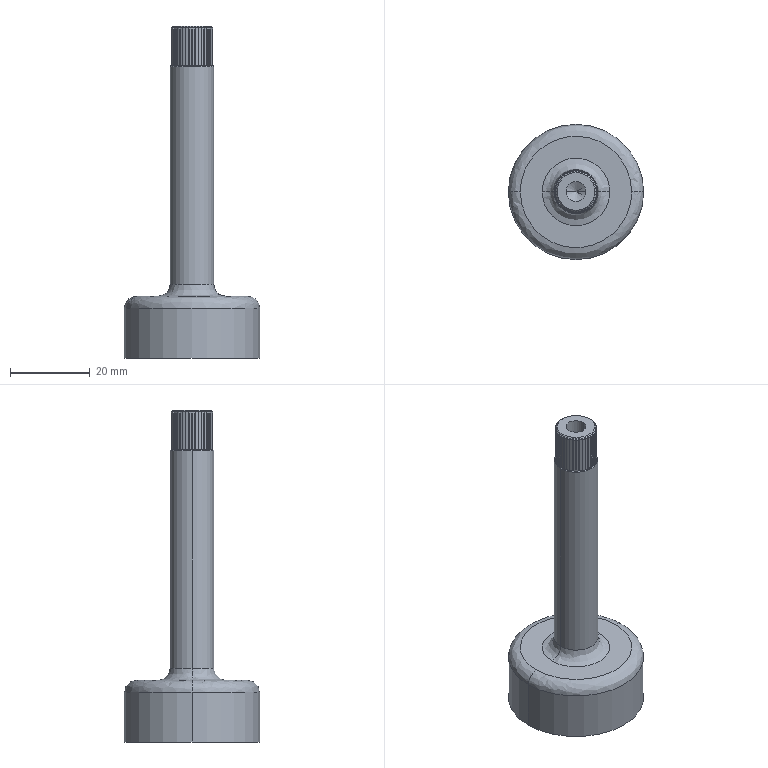Part | STEP file | Product lower | 1 solid | 185 faces | box 34 x 34 x 83.5 mm | volume 10000 mm3 | plane 125 | cylinder 48 | cone 8 | spline 4 | commonest cylinder face diameters 10.5 x40 5 x2 11 x2 30 x2 34 x2